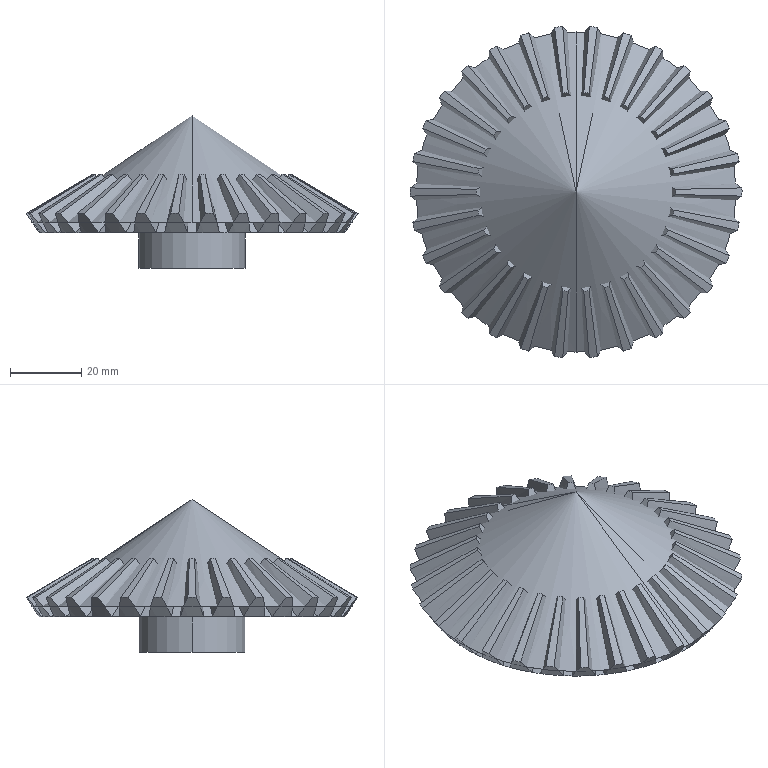Part | SolidWorks | 1 solid | 195 faces | box 93.328 x 93.03 x 42.995 mm | volume 13757 mm3 | cone 123 | spline 60 | plane 7 | cylinder 5 | commonest cylinder face diameters 20 x3 30 x2